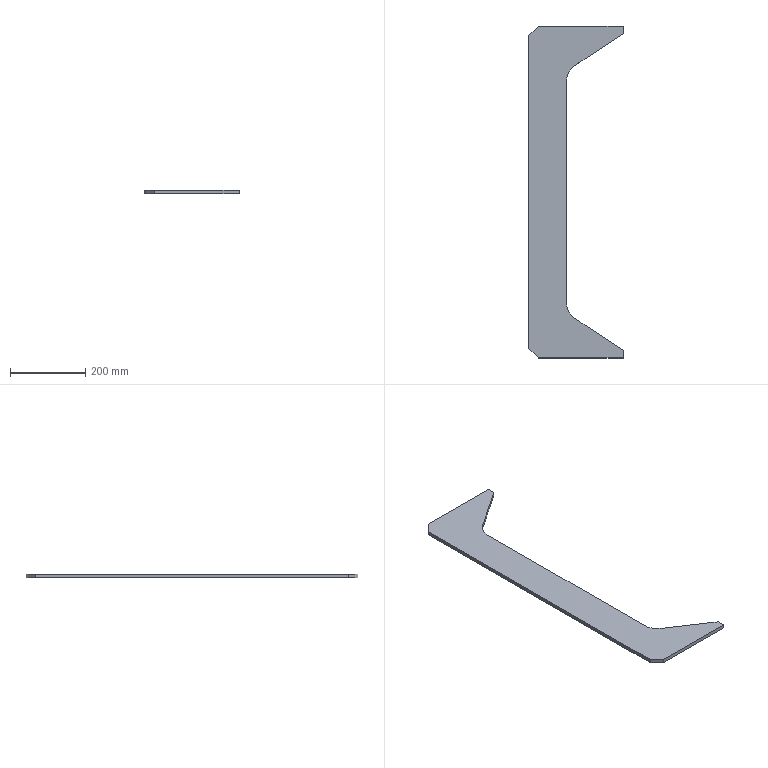Part | SolidWorks | features Chamfer 1, Extrusion 1, Fillet 1 | 1 solid | 14 faces | box 250 x 880 x 10 mm | volume 1085939 mm3 | plane 12 | cylinder 2 | commonest cylinder face diameters 100 x2
STEP:
#1=CARTESIAN_POINT('',(-25.,440.,0.));
#2=VERTEX_POINT('',#1);
#3=CARTESIAN_POINT('',(200.,440.,0.));
#4=VERTEX_POINT('',#3);
#5=CARTESIAN_POINT('',(0.,440.,0.));
#6=DIRECTION('',(1.,0.,0.));
#7=VECTOR('',#6,1000.);
#8=LINE('',#5,#7);
#9=EDGE_CURVE('',#2,#4,#8,.T.);
#10=ORIENTED_EDGE('',*,*,#9,.F.);
#11=CARTESIAN_POINT('',(-25.,440.,10.));
#12=VERTEX_POINT('',#11);
#13=CARTESIAN_POINT('',(-25.,440.,10.));
#14=DIRECTION('',(0.,0.,1.));
#15=VECTOR('',#14,1000.);
#16=LINE('',#13,#15);
#17=EDGE_CURVE('',#2,#12,#16,.T.);
#18=ORIENTED_EDGE('',*,*,#17,.T.);
#19=CARTESIAN_POINT('',(200.,440.,10.));
#20=VERTEX_POINT('',#19);
#21=CARTESIAN_POINT('',(0.,440.,10.));
#22=DIRECTION('',(1.,0.,0.));
#23=VECTOR('',#22,1000.);
#24=LINE('',#21,#23);
#25=EDGE_CURVE('',#12,#20,#24,.T.);
#26=ORIENTED_EDGE('',*,*,#25,.T.);
#27=CARTESIAN_POINT('',(200.,440.,10.));
#28=DIRECTION('',(0.,0.,-1.));
#29=VECTOR('',#28,1000.);
#30=LINE('',#27,#29);
#31=EDGE_CURVE('',#20,#4,#30,.T.);
#32=ORIENTED_EDGE('',*,*,#31,.T.);
#33=EDGE_LOOP('',(#10,#18,#26,#32));
#34=FACE_OUTER_BOUND('',#33,.T.);
#35=CARTESIAN_POINT('',(0.,440.,10.));
#36=DIRECTION('',(0.,1.,0.));
#37=DIRECTION('',(0.,0.,1.));
#38=AXIS2_PLACEMENT_3D('',#35,#36,#37);
#39=PLANE('',#38);
#40=ADVANCED_FACE('',(#34),#39,.T.);
#41=CARTESIAN_POINT('',(-50.,-415.,10.));
#42=VERTEX_POINT('',#41);
#43=CARTESIAN_POINT('',(-50.,415.,10.));
#44=VERTEX_POINT('',#43);
#45=CARTESIAN_POINT('',(-50.,0.,10.));
#46=DIRECTION('',(0.,1.,0.));
#47=VECTOR('',#46,1000.);
#48=LINE('',#45,#47);
#49=EDGE_CURVE('',#42,#44,#48,.T.);
#50=ORIENTED_EDGE('',*,*,#49,.T.);
#51=CARTESIAN_POINT('',(-50.,415.,0.));
#52=VERTEX_POINT('',#51);
#53=CARTESIAN_POINT('',(-50.,415.,10.));
#54=DIRECTION('',(0.,0.,-1.));
#55=VECTOR('',#54,1000.);
#56=LINE('',#53,#55);
#57=EDGE_CURVE('',#44,#52,#56,.T.);
#58=ORIENTED_EDGE('',*,*,#57,.T.);
#59=CARTESIAN_POINT('',(-50.,-415.,0.));
#60=VERTEX_POINT('',#59);
#61=CARTESIAN_POINT('',(-50.,0.,0.));
#62=DIRECTION('',(0.,1.,0.));
#63=VECTOR('',#62,1000.);
#64=LINE('',#61,#63);
#65=EDGE_CURVE('',#60,#52,#64,.T.);
#66=ORIENTED_EDGE('',*,*,#65,.F.);
#67=CARTESIAN_POINT('',(-50.,-415.,10.));
#68=DIRECTION('',(0.,0.,1.));
#69=VECTOR('',#68,1000.);
#70=LINE('',#67,#69);
#71=EDGE_CURVE('',#60,#42,#70,.T.);
#72=ORIENTED_EDGE('',*,*,#71,.T.);
#73=EDGE_LOOP('',(#50,#58,#66,#72));
#74=FACE_OUTER_BOUND('',#73,.T.);
#75=CARTESIAN_POINT('',(-50.,0.,10.));
#76=DIRECTION('',(-1.,0.,0.));
#77=DIRECTION('',(0.,0.,1.));
#78=AXIS2_PLACEMENT_3D('',#75,#76,#77);
#79=PLANE('',#78);
#80=ADVANCED_FACE('',(#74),#79,.T.);
#81=CARTESIAN_POINT('',(-25.,-440.,10.));
#82=VERTEX_POINT('',#81);
#83=CARTESIAN_POINT('',(200.,-440.,10.));
#84=VERTEX_POINT('',#83);
#85=CARTESIAN_POINT('',(0.,-440.,10.));
#86=DIRECTION('',(1.,0.,0.));
#87=VECTOR('',#86,1000.);
#88=LINE('',#85,#87);
#89=EDGE_CURVE('',#82,#84,#88,.T.);
#90=ORIENTED_EDGE('',*,*,#89,.F.);
#91=CARTESIAN_POINT('',(-25.,-440.,0.));
#92=VERTEX_POINT('',#91);
#93=CARTESIAN_POINT('',(-25.,-440.,0.));
#94=DIRECTION('',(0.,0.,-1.));
#95=VECTOR('',#94,1000.);
#96=LINE('',#93,#95);
#97=EDGE_CURVE('',#82,#92,#96,.T.);
#98=ORIENTED_EDGE('',*,*,#97,.T.);
#99=CARTESIAN_POINT('',(200.,-440.,0.));
#100=VERTEX_POINT('',#99);
#101=CARTESIAN_POINT('',(0.,-440.,0.));
#102=DIRECTION('',(1.,0.,0.));
#103=VECTOR('',#102,1000.);
#104=LINE('',#101,#103);
#105=EDGE_CURVE('',#92,#100,#104,.T.);
#106=ORIENTED_EDGE('',*,*,#105,.T.);
#107=CARTESIAN_POINT('',(200.,-440.,10.));
#108=DIRECTION('',(0.,0.,-1.));
#109=VECTOR('',#108,1000.);
#110=LINE('',#107,#109);
#111=EDGE_CURVE('',#84,#100,#110,.T.);
#112=ORIENTED_EDGE('',*,*,#111,.F.);
#113=EDGE_LOOP('',(#90,#98,#106,#112));
#114=FACE_OUTER_BOUND('',#113,.T.);
#115=CARTESIAN_POINT('',(0.,-440.,10.));
#116=DIRECTION('',(0.,1.,0.));
#117=DIRECTION('',(0.,0.,1.));
#118=AXIS2_PLACEMENT_3D('',#115,#116,#117);
#119=PLANE('',#118);
#120=ADVANCED_FACE('',(#114),#119,.F.);
#121=CARTESIAN_POINT('',(200.,-420.,0.));
#122=VERTEX_POINT('',#121);
#123=CARTESIAN_POINT('',(200.,0.,0.));
#124=DIRECTION('',(0.,1.,0.));
#125=VECTOR('',#124,1000.);
#126=LINE('',#123,#125);
#127=EDGE_CURVE('',#100,#122,#126,.T.);
#128=ORIENTED_EDGE('',*,*,#127,.T.);
#129=CARTESIAN_POINT('',(200.,-420.,10.));
#130=VERTEX_POINT('',#129);
#131=CARTESIAN_POINT('',(200.,-420.,10.));
#132=DIRECTION('',(0.,0.,-1.));
#133=VECTOR('',#132,1000.);
#134=LINE('',#131,#133);
#135=EDGE_CURVE('',#130,#122,#134,.T.);
#136=ORIENTED_EDGE('',*,*,#135,.F.);
#137=CARTESIAN_POINT('',(200.,0.,10.));
#138=DIRECTION('',(0.,1.,0.));
#139=VECTOR('',#138,1000.);
#140=LINE('',#137,#139);
#141=EDGE_CURVE('',#84,#130,#140,.T.);
#142=ORIENTED_EDGE('',*,*,#141,.F.);
#143=ORIENTED_EDGE('',*,*,#111,.T.);
#144=EDGE_LOOP('',(#128,#136,#142,#143));
#145=FACE_OUTER_BOUND('',#144,.T.);
#146=CARTESIAN_POINT('',(200.,0.,10.));
#147=DIRECTION('',(-1.,0.,0.));
#148=DIRECTION('',(0.,0.,1.));
#149=AXIS2_PLACEMENT_3D('',#146,#147,#148);
#150=PLANE('',#149);
#151=ADVANCED_FACE('',(#145),#150,.F.);
#152=CARTESIAN_POINT('',(72.265,-334.843,0.));
#153=VERTEX_POINT('',#152);
#154=CARTESIAN_POINT('',(-132.308,-198.462,0.));
#155=DIRECTION('',(-0.8321,0.5547,0.));
#156=VECTOR('',#155,1000.);
#157=LINE('',#154,#156);
#158=EDGE_CURVE('',#122,#153,#157,.T.);
#159=ORIENTED_EDGE('',*,*,#158,.T.);
#160=CARTESIAN_POINT('',(72.265,-334.843,10.));
#161=VERTEX_POINT('',#160);
#162=CARTESIAN_POINT('',(72.265,-334.843,10.));
#163=DIRECTION('',(0.,0.,1.));
#164=VECTOR('',#163,1000.);
#165=LINE('',#162,#164);
#166=EDGE_CURVE('',#153,#161,#165,.T.);
#167=ORIENTED_EDGE('',*,*,#166,.T.);
#168=CARTESIAN_POINT('',(-132.308,-198.462,10.));
#169=DIRECTION('',(-0.8321,0.5547,0.));
#170=VECTOR('',#169,1000.);
#171=LINE('',#168,#170);
#172=EDGE_CURVE('',#130,#161,#171,.T.);
#173=ORIENTED_EDGE('',*,*,#172,.F.);
#174=ORIENTED_EDGE('',*,*,#135,.T.);
#175=EDGE_LOOP('',(#159,#167,#173,#174));
#176=FACE_OUTER_BOUND('',#175,.T.);
#177=CARTESIAN_POINT('',(-132.308,-198.462,10.));
#178=DIRECTION('',(-0.5547,-0.8321,0.));
#179=DIRECTION('',(0.8321,-0.5547,0.));
#180=AXIS2_PLACEMENT_3D('',#177,#178,#179);
#181=PLANE('',#180);
#182=ADVANCED_FACE('',(#176),#181,.F.);
#183=CARTESIAN_POINT('',(50.,-293.241,10.));
#184=VERTEX_POINT('',#183);
#185=CARTESIAN_POINT('',(50.,293.241,10.));
#186=VERTEX_POINT('',#185);
#187=CARTESIAN_POINT('',(50.,0.,10.));
#188=DIRECTION('',(0.,1.,0.));
#189=VECTOR('',#188,1000.);
#190=LINE('',#187,#189);
#191=EDGE_CURVE('',#184,#186,#190,.T.);
#192=ORIENTED_EDGE('',*,*,#191,.F.);
#193=CARTESIAN_POINT('',(50.,-293.241,0.));
#194=VERTEX_POINT('',#193);
#195=CARTESIAN_POINT('',(50.,-293.241,0.));
#196=DIRECTION('',(0.,0.,-1.));
#197=VECTOR('',#196,1000.);
#198=LINE('',#195,#197);
#199=EDGE_CURVE('',#184,#194,#198,.T.);
#200=ORIENTED_EDGE('',*,*,#199,.T.);
#201=CARTESIAN_POINT('',(50.,293.241,0.));
#202=VERTEX_POINT('',#201);
#203=CARTESIAN_POINT('',(50.,0.,0.));
#204=DIRECTION('',(0.,1.,0.));
#205=VECTOR('',#204,1000.);
#206=LINE('',#203,#205);
#207=EDGE_CURVE('',#194,#202,#206,.T.);
#208=ORIENTED_EDGE('',*,*,#207,.T.);
#209=CARTESIAN_POINT('',(50.,293.241,10.));
#210=DIRECTION('',(0.,0.,1.));
#211=VECTOR('',#210,1000.);
#212=LINE('',#209,#211);
#213=EDGE_CURVE('',#202,#186,#212,.T.);
#214=ORIENTED_EDGE('',*,*,#213,.T.);
#215=EDGE_LOOP('',(#192,#200,#208,#214));
#216=FACE_OUTER_BOUND('',#215,.T.);
#217=CARTESIAN_POINT('',(50.,0.,10.));
#218=DIRECTION('',(-1.,0.,0.));
#219=DIRECTION('',(0.,0.,1.));
#220=AXIS2_PLACEMENT_3D('',#217,#218,#219);
#221=PLANE('',#220);
#222=ADVANCED_FACE('',(#216),#221,.F.);
#223=CARTESIAN_POINT('',(200.,420.,10.));
#224=VERTEX_POINT('',#223);
#225=CARTESIAN_POINT('',(72.265,334.843,10.));
#226=VERTEX_POINT('',#225);
#227=CARTESIAN_POINT('',(-132.308,198.462,10.));
#228=DIRECTION('',(-0.8321,-0.5547,0.));
#229=VECTOR('',#228,1000.);
#230=LINE('',#227,#229);
#231=EDGE_CURVE('',#224,#226,#230,.T.);
#232=ORIENTED_EDGE('',*,*,#231,.T.);
#233=CARTESIAN_POINT('',(72.265,334.843,0.));
#234=VERTEX_POINT('',#233);
#235=CARTESIAN_POINT('',(72.265,334.843,10.));
#236=DIRECTION('',(0.,0.,-1.));
#237=VECTOR('',#236,1000.);
#238=LINE('',#235,#237);
#239=EDGE_CURVE('',#226,#234,#238,.T.);
#240=ORIENTED_EDGE('',*,*,#239,.T.);
#241=CARTESIAN_POINT('',(200.,420.,0.));
#242=VERTEX_POINT('',#241);
#243=CARTESIAN_POINT('',(-132.308,198.462,0.));
#244=DIRECTION('',(-0.8321,-0.5547,0.));
#245=VECTOR('',#244,1000.);
#246=LINE('',#243,#245);
#247=EDGE_CURVE('',#242,#234,#246,.T.);
#248=ORIENTED_EDGE('',*,*,#247,.F.);
#249=CARTESIAN_POINT('',(200.,420.,10.));
#250=DIRECTION('',(0.,0.,-1.));
#251=VECTOR('',#250,1000.);
#252=LINE('',#249,#251);
#253=EDGE_CURVE('',#224,#242,#252,.T.);
#254=ORIENTED_EDGE('',*,*,#253,.F.);
#255=EDGE_LOOP('',(#232,#240,#248,#254));
#256=FACE_OUTER_BOUND('',#255,.T.);
#257=CARTESIAN_POINT('',(-132.308,198.462,10.));
#258=DIRECTION('',(0.5547,-0.8321,0.));
#259=DIRECTION('',(0.8321,0.5547,0.));
#260=AXIS2_PLACEMENT_3D('',#257,#258,#259);
#261=PLANE('',#260);
#262=ADVANCED_FACE('',(#256),#261,.T.);
#263=CARTESIAN_POINT('',(200.,0.,0.));
#264=DIRECTION('',(0.,-1.,0.));
#265=VECTOR('',#264,1000.);
#266=LINE('',#263,#265);
#267=EDGE_CURVE('',#4,#242,#266,.T.);
#268=ORIENTED_EDGE('',*,*,#267,.F.);
#269=ORIENTED_EDGE('',*,*,#31,.F.);
#270=CARTESIAN_POINT('',(200.,0.,10.));
#271=DIRECTION('',(0.,-1.,0.));
#272=VECTOR('',#271,1000.);
#273=LINE('',#270,#272);
#274=EDGE_CURVE('',#20,#224,#273,.T.);
#275=ORIENTED_EDGE('',*,*,#274,.T.);
#276=ORIENTED_EDGE('',*,*,#253,.T.);
#277=EDGE_LOOP('',(#268,#269,#275,#276));
#278=FACE_OUTER_BOUND('',#277,.T.);
#279=CARTESIAN_POINT('',(200.,0.,10.));
#280=DIRECTION('',(1.,0.,0.));
#281=DIRECTION('',(0.,0.,-1.));
#282=AXIS2_PLACEMENT_3D('',#279,#280,#281);
#283=PLANE('',#282);
#284=ADVANCED_FACE('',(#278),#283,.T.);
#285=ORIENTED_EDGE('',*,*,#25,.F.);
#286=CARTESIAN_POINT('',(-232.5,232.5,10.));
#287=DIRECTION('',(-0.7071,-0.7071,0.));
#288=VECTOR('',#287,1000.);
#289=LINE('',#286,#288);
#290=EDGE_CURVE('',#12,#44,#289,.T.);
#291=ORIENTED_EDGE('',*,*,#290,.T.);
#292=ORIENTED_EDGE('',*,*,#49,.F.);
#293=CARTESIAN_POINT('',(-232.5,-232.5,10.));
#294=DIRECTION('',(0.7071,-0.7071,0.));
#295=VECTOR('',#294,1000.);
#296=LINE('',#293,#295);
#297=EDGE_CURVE('',#42,#82,#296,.T.);
#298=ORIENTED_EDGE('',*,*,#297,.T.);
#299=ORIENTED_EDGE('',*,*,#89,.T.);
#300=ORIENTED_EDGE('',*,*,#141,.T.);
#301=ORIENTED_EDGE('',*,*,#172,.T.);
#302=CARTESIAN_POINT('',(100.,-293.241,10.));
#303=DIRECTION('',(0.,0.,-1.));
#304=DIRECTION('',(1.,0.,0.));
#305=AXIS2_PLACEMENT_3D('',#302,#303,#304);
#306=CIRCLE('',#305,50.);
#307=EDGE_CURVE('',#161,#184,#306,.T.);
#308=ORIENTED_EDGE('',*,*,#307,.T.);
#309=ORIENTED_EDGE('',*,*,#191,.T.);
#310=CARTESIAN_POINT('',(100.,293.241,10.));
#311=DIRECTION('',(0.,0.,-1.));
#312=DIRECTION('',(1.,0.,0.));
#313=AXIS2_PLACEMENT_3D('',#310,#311,#312);
#314=CIRCLE('',#313,50.);
#315=EDGE_CURVE('',#186,#226,#314,.T.);
#316=ORIENTED_EDGE('',*,*,#315,.T.);
#317=ORIENTED_EDGE('',*,*,#231,.F.);
#318=ORIENTED_EDGE('',*,*,#274,.F.);
#319=EDGE_LOOP('',(#285,#291,#292,#298,#299,#300,#301,#308,#309,#316,#317,#318));
#320=FACE_OUTER_BOUND('',#319,.T.);
#321=CARTESIAN_POINT('',(0.,0.,10.));
#322=DIRECTION('',(0.,0.,1.));
#323=DIRECTION('',(1.,0.,0.));
#324=AXIS2_PLACEMENT_3D('',#321,#322,#323);
#325=PLANE('',#324);
#326=ADVANCED_FACE('',(#320),#325,.T.);
#327=ORIENTED_EDGE('',*,*,#65,.T.);
#328=CARTESIAN_POINT('',(-50.,415.,0.));
#329=DIRECTION('',(0.7071,0.7071,0.));
#330=VECTOR('',#329,1000.);
#331=LINE('',#328,#330);
#332=EDGE_CURVE('',#52,#2,#331,.T.);
#333=ORIENTED_EDGE('',*,*,#332,.T.);
#334=ORIENTED_EDGE('',*,*,#9,.T.);
#335=ORIENTED_EDGE('',*,*,#267,.T.);
#336=ORIENTED_EDGE('',*,*,#247,.T.);
#337=CARTESIAN_POINT('',(100.,293.241,0.));
#338=DIRECTION('',(0.,0.,1.));
#339=DIRECTION('',(1.,0.,0.));
#340=AXIS2_PLACEMENT_3D('',#337,#338,#339);
#341=CIRCLE('',#340,50.);
#342=EDGE_CURVE('',#234,#202,#341,.T.);
#343=ORIENTED_EDGE('',*,*,#342,.T.);
#344=ORIENTED_EDGE('',*,*,#207,.F.);
#345=CARTESIAN_POINT('',(100.,-293.241,0.));
#346=DIRECTION('',(0.,0.,1.));
#347=DIRECTION('',(1.,0.,0.));
#348=AXIS2_PLACEMENT_3D('',#345,#346,#347);
#349=CIRCLE('',#348,50.);
#350=EDGE_CURVE('',#194,#153,#349,.T.);
#351=ORIENTED_EDGE('',*,*,#350,.T.);
#352=ORIENTED_EDGE('',*,*,#158,.F.);
#353=ORIENTED_EDGE('',*,*,#127,.F.);
#354=ORIENTED_EDGE('',*,*,#105,.F.);
#355=CARTESIAN_POINT('',(-25.,-440.,0.));
#356=DIRECTION('',(-0.7071,0.7071,0.));
#357=VECTOR('',#356,1000.);
#358=LINE('',#355,#357);
#359=EDGE_CURVE('',#92,#60,#358,.T.);
#360=ORIENTED_EDGE('',*,*,#359,.T.);
#361=EDGE_LOOP('',(#327,#333,#334,#335,#336,#343,#344,#351,#352,#353,#354,#360));
#362=FACE_OUTER_BOUND('',#361,.T.);
#363=CARTESIAN_POINT('',(0.,0.,0.));
#364=DIRECTION('',(0.,0.,1.));
#365=DIRECTION('',(1.,0.,0.));
#366=AXIS2_PLACEMENT_3D('',#363,#364,#365);
#367=PLANE('',#366);
#368=ADVANCED_FACE('',(#362),#367,.F.);
#369=ORIENTED_EDGE('',*,*,#307,.F.);
#370=ORIENTED_EDGE('',*,*,#166,.F.);
#371=ORIENTED_EDGE('',*,*,#350,.F.);
#372=ORIENTED_EDGE('',*,*,#199,.F.);
#373=EDGE_LOOP('',(#369,#370,#371,#372));
#374=FACE_OUTER_BOUND('',#373,.T.);
#375=CARTESIAN_POINT('',(100.,-293.241,10.));
#376=DIRECTION('',(0.,0.,1.));
#377=DIRECTION('',(1.,0.,0.));
#378=AXIS2_PLACEMENT_3D('',#375,#376,#377);
#379=CYLINDRICAL_SURFACE('',#378,50.);
#380=ADVANCED_FACE('',(#374),#379,.F.);
#381=ORIENTED_EDGE('',*,*,#315,.F.);
#382=ORIENTED_EDGE('',*,*,#213,.F.);
#383=ORIENTED_EDGE('',*,*,#342,.F.);
#384=ORIENTED_EDGE('',*,*,#239,.F.);
#385=EDGE_LOOP('',(#381,#382,#383,#384));
#386=FACE_OUTER_BOUND('',#385,.T.);
#387=CARTESIAN_POINT('',(100.,293.241,10.));
#388=DIRECTION('',(0.,0.,-1.));
#389=DIRECTION('',(-1.,0.,0.));
#390=AXIS2_PLACEMENT_3D('',#387,#388,#389);
#391=CYLINDRICAL_SURFACE('',#390,50.);
#392=ADVANCED_FACE('',(#386),#391,.F.);
#393=ORIENTED_EDGE('',*,*,#290,.F.);
#394=ORIENTED_EDGE('',*,*,#17,.F.);
#395=ORIENTED_EDGE('',*,*,#332,.F.);
#396=ORIENTED_EDGE('',*,*,#57,.F.);
#397=EDGE_LOOP('',(#393,#394,#395,#396));
#398=FACE_OUTER_BOUND('',#397,.T.);
#399=CARTESIAN_POINT('',(-50.,415.,10.));
#400=DIRECTION('',(0.7071,-0.7071,0.));
#401=DIRECTION('',(0.,0.,-1.));
#402=AXIS2_PLACEMENT_3D('',#399,#400,#401);
#403=PLANE('',#402);
#404=ADVANCED_FACE('',(#398),#403,.F.);
#405=ORIENTED_EDGE('',*,*,#297,.F.);
#406=ORIENTED_EDGE('',*,*,#71,.F.);
#407=ORIENTED_EDGE('',*,*,#359,.F.);
#408=ORIENTED_EDGE('',*,*,#97,.F.);
#409=EDGE_LOOP('',(#405,#406,#407,#408));
#410=FACE_OUTER_BOUND('',#409,.T.);
#411=CARTESIAN_POINT('',(-25.,-440.,10.));
#412=DIRECTION('',(-0.7071,-0.7071,0.));
#413=DIRECTION('',(0.,0.,1.));
#414=AXIS2_PLACEMENT_3D('',#411,#412,#413);
#415=PLANE('',#414);
#416=ADVANCED_FACE('',(#410),#415,.T.);
#417=CLOSED_SHELL('',(#40,#80,#120,#151,#182,#222,#262,#284,#326,#368,#380,#392,#404,#416));
#418=MANIFOLD_SOLID_BREP('',#417);
#419=CARTESIAN_POINT('',(0.,0.,0.));
#420=DIRECTION('',(0.,0.,1.));
#421=DIRECTION('',(1.,0.,0.));
#422=AXIS2_PLACEMENT_3D('',#419,#420,#421);
#423=(LENGTH_UNIT()NAMED_UNIT(*)SI_UNIT(.MILLI.,.METRE.));
#424=UNCERTAINTY_MEASURE_WITH_UNIT(LENGTH_MEASURE(0.00001),#423,'','');
#425=(NAMED_UNIT(*)PLANE_ANGLE_UNIT()SI_UNIT($,.RADIAN.));
#426=(NAMED_UNIT(*)SI_UNIT($,.STERADIAN.)SOLID_ANGLE_UNIT());
#427=(GEOMETRIC_REPRESENTATION_CONTEXT(3)GLOBAL_UNCERTAINTY_ASSIGNED_CONTEXT((#424))GLOBAL_UNIT_ASSIGNED_CONTEXT((#423,#425,#426))REPRESENTATION_CONTEXT('',''));
#428=ADVANCED_BREP_SHAPE_REPRESENTATION('',(#418,#422),#427);